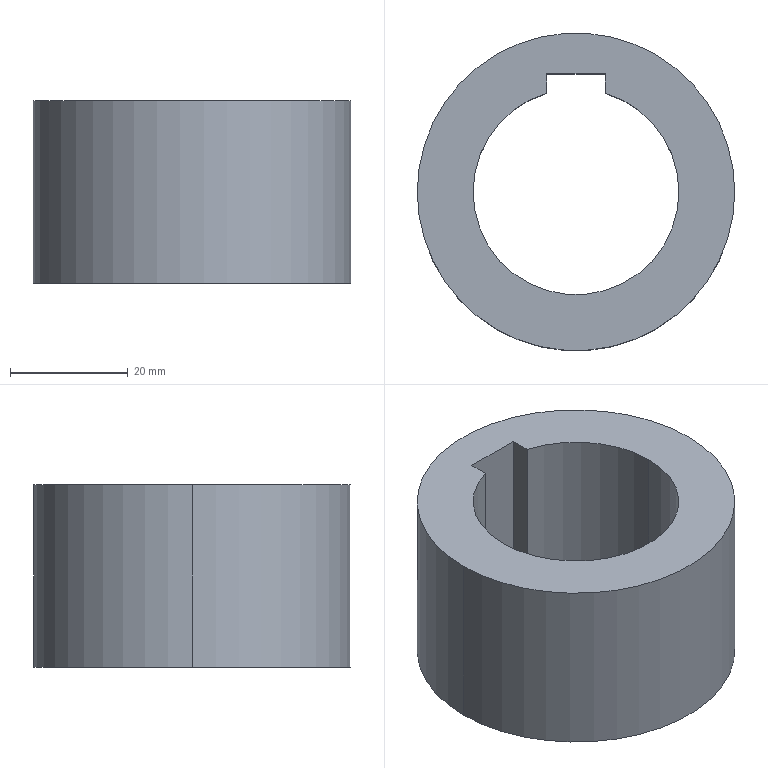Part | SolidWorks | features ICE 3, CirPattern 1, Extrusion 1, RefAxis 1 | 1 solid | 10 faces | box 54 x 54 x 31 mm | volume 40300 mm3 | cylinder 5 | plane 5 | commonest cylinder face diameters 35 x3 54 x2
STEP:
#1=CARTESIAN_POINT('',(-27.,0.,31.));
#2=VERTEX_POINT('',#1);
#3=CARTESIAN_POINT('',(27.,0.,31.));
#4=VERTEX_POINT('',#3);
#5=CARTESIAN_POINT('',(0.,0.,31.));
#6=DIRECTION('',(0.,0.,-1.));
#7=DIRECTION('',(1.,0.,0.));
#8=AXIS2_PLACEMENT_3D('',#5,#6,#7);
#9=CIRCLE('',#8,27.);
#10=EDGE_CURVE('',#2,#4,#9,.T.);
#11=ORIENTED_EDGE('',*,*,#10,.T.);
#12=CARTESIAN_POINT('',(27.,0.,0.));
#13=VERTEX_POINT('',#12);
#14=CARTESIAN_POINT('',(27.,0.,42.));
#15=DIRECTION('',(0.,0.,-1.));
#16=VECTOR('',#15,1000.);
#17=LINE('',#14,#16);
#18=EDGE_CURVE('',#4,#13,#17,.T.);
#19=ORIENTED_EDGE('',*,*,#18,.T.);
#20=CARTESIAN_POINT('',(-27.,0.,0.));
#21=VERTEX_POINT('',#20);
#22=CARTESIAN_POINT('',(0.,0.,0.));
#23=DIRECTION('',(0.,0.,1.));
#24=DIRECTION('',(1.,0.,0.));
#25=AXIS2_PLACEMENT_3D('',#22,#23,#24);
#26=CIRCLE('',#25,27.);
#27=EDGE_CURVE('',#13,#21,#26,.T.);
#28=ORIENTED_EDGE('',*,*,#27,.T.);
#29=CARTESIAN_POINT('',(-27.,0.,42.));
#30=DIRECTION('',(0.,0.,-1.));
#31=VECTOR('',#30,1000.);
#32=LINE('',#29,#31);
#33=EDGE_CURVE('',#2,#21,#32,.T.);
#34=ORIENTED_EDGE('',*,*,#33,.F.);
#35=EDGE_LOOP('',(#11,#19,#28,#34));
#36=FACE_OUTER_BOUND('',#35,.T.);
#37=CARTESIAN_POINT('',(0.,0.,42.));
#38=DIRECTION('',(0.,0.,-1.));
#39=DIRECTION('',(-1.,0.,0.));
#40=AXIS2_PLACEMENT_3D('',#37,#38,#39);
#41=CYLINDRICAL_SURFACE('',#40,27.);
#42=ADVANCED_FACE('',(#36),#41,.T.);
#43=CARTESIAN_POINT('',(-17.5,0.,0.));
#44=VERTEX_POINT('',#43);
#45=CARTESIAN_POINT('',(17.5,0.,0.));
#46=VERTEX_POINT('',#45);
#47=CARTESIAN_POINT('',(0.,0.,0.));
#48=DIRECTION('',(0.,0.,1.));
#49=DIRECTION('',(1.,0.,0.));
#50=AXIS2_PLACEMENT_3D('',#47,#48,#49);
#51=CIRCLE('',#50,17.5);
#52=EDGE_CURVE('',#44,#46,#51,.T.);
#53=ORIENTED_EDGE('',*,*,#52,.F.);
#54=CARTESIAN_POINT('',(-17.5,0.,31.));
#55=VERTEX_POINT('',#54);
#56=CARTESIAN_POINT('',(-17.5,0.,0.));
#57=DIRECTION('',(0.,0.,1.));
#58=VECTOR('',#57,1000.);
#59=LINE('',#56,#58);
#60=EDGE_CURVE('',#44,#55,#59,.T.);
#61=ORIENTED_EDGE('',*,*,#60,.T.);
#62=CARTESIAN_POINT('',(17.5,0.,31.));
#63=VERTEX_POINT('',#62);
#64=CARTESIAN_POINT('',(0.,0.,31.));
#65=DIRECTION('',(0.,0.,1.));
#66=DIRECTION('',(1.,0.,0.));
#67=AXIS2_PLACEMENT_3D('',#64,#65,#66);
#68=CIRCLE('',#67,17.5);
#69=EDGE_CURVE('',#55,#63,#68,.T.);
#70=ORIENTED_EDGE('',*,*,#69,.T.);
#71=CARTESIAN_POINT('',(17.5,0.,0.));
#72=DIRECTION('',(0.,0.,1.));
#73=VECTOR('',#72,1000.);
#74=LINE('',#71,#73);
#75=EDGE_CURVE('',#46,#63,#74,.T.);
#76=ORIENTED_EDGE('',*,*,#75,.F.);
#77=EDGE_LOOP('',(#53,#61,#70,#76));
#78=FACE_OUTER_BOUND('',#77,.T.);
#79=CARTESIAN_POINT('',(0.,0.,0.));
#80=DIRECTION('',(0.,0.,1.));
#81=DIRECTION('',(1.,0.,0.));
#82=AXIS2_PLACEMENT_3D('',#79,#80,#81);
#83=CYLINDRICAL_SURFACE('',#82,17.5);
#84=ADVANCED_FACE('',(#78),#83,.F.);
#85=CARTESIAN_POINT('',(5.,16.771,0.));
#86=VERTEX_POINT('',#85);
#87=CARTESIAN_POINT('',(0.,0.,0.));
#88=DIRECTION('',(0.,0.,1.));
#89=DIRECTION('',(1.,0.,0.));
#90=AXIS2_PLACEMENT_3D('',#87,#88,#89);
#91=CIRCLE('',#90,17.5);
#92=EDGE_CURVE('',#46,#86,#91,.T.);
#93=ORIENTED_EDGE('',*,*,#92,.F.);
#94=ORIENTED_EDGE('',*,*,#75,.T.);
#95=CARTESIAN_POINT('',(5.,16.771,31.));
#96=VERTEX_POINT('',#95);
#97=CARTESIAN_POINT('',(0.,0.,31.));
#98=DIRECTION('',(0.,0.,1.));
#99=DIRECTION('',(1.,0.,0.));
#100=AXIS2_PLACEMENT_3D('',#97,#98,#99);
#101=CIRCLE('',#100,17.5);
#102=EDGE_CURVE('',#63,#96,#101,.T.);
#103=ORIENTED_EDGE('',*,*,#102,.T.);
#104=CARTESIAN_POINT('',(5.,16.771,0.));
#105=DIRECTION('',(0.,0.,1.));
#106=VECTOR('',#105,1000.);
#107=LINE('',#104,#106);
#108=EDGE_CURVE('',#86,#96,#107,.T.);
#109=ORIENTED_EDGE('',*,*,#108,.F.);
#110=EDGE_LOOP('',(#93,#94,#103,#109));
#111=FACE_OUTER_BOUND('',#110,.T.);
#112=CARTESIAN_POINT('',(0.,0.,0.));
#113=DIRECTION('',(0.,0.,1.));
#114=DIRECTION('',(1.,0.,0.));
#115=AXIS2_PLACEMENT_3D('',#112,#113,#114);
#116=CYLINDRICAL_SURFACE('',#115,17.5);
#117=ADVANCED_FACE('',(#111),#116,.F.);
#118=CARTESIAN_POINT('',(-5.,16.771,31.));
#119=VERTEX_POINT('',#118);
#120=CARTESIAN_POINT('',(0.,0.,31.));
#121=DIRECTION('',(0.,0.,1.));
#122=DIRECTION('',(1.,0.,0.));
#123=AXIS2_PLACEMENT_3D('',#120,#121,#122);
#124=CIRCLE('',#123,17.5);
#125=EDGE_CURVE('',#119,#55,#124,.T.);
#126=ORIENTED_EDGE('',*,*,#125,.F.);
#127=CARTESIAN_POINT('',(-5.,20.071,31.));
#128=VERTEX_POINT('',#127);
#129=CARTESIAN_POINT('',(-5.,20.071,31.));
#130=DIRECTION('',(0.,-1.,0.));
#131=VECTOR('',#130,1000.);
#132=LINE('',#129,#131);
#133=EDGE_CURVE('',#128,#119,#132,.T.);
#134=ORIENTED_EDGE('',*,*,#133,.F.);
#135=CARTESIAN_POINT('',(5.,20.071,31.));
#136=VERTEX_POINT('',#135);
#137=CARTESIAN_POINT('',(5.,20.071,31.));
#138=DIRECTION('',(-1.,0.,0.));
#139=VECTOR('',#138,1000.);
#140=LINE('',#137,#139);
#141=EDGE_CURVE('',#136,#128,#140,.T.);
#142=ORIENTED_EDGE('',*,*,#141,.F.);
#143=CARTESIAN_POINT('',(5.,16.771,31.));
#144=DIRECTION('',(0.,1.,0.));
#145=VECTOR('',#144,1000.);
#146=LINE('',#143,#145);
#147=EDGE_CURVE('',#96,#136,#146,.T.);
#148=ORIENTED_EDGE('',*,*,#147,.F.);
#149=ORIENTED_EDGE('',*,*,#102,.F.);
#150=ORIENTED_EDGE('',*,*,#69,.F.);
#151=EDGE_LOOP('',(#126,#134,#142,#148,#149,#150));
#152=FACE_BOUND('',#151,.T.);
#153=ORIENTED_EDGE('',*,*,#10,.F.);
#154=CARTESIAN_POINT('',(0.,0.,31.));
#155=DIRECTION('',(0.,0.,-1.));
#156=DIRECTION('',(1.,0.,0.));
#157=AXIS2_PLACEMENT_3D('',#154,#155,#156);
#158=CIRCLE('',#157,27.);
#159=EDGE_CURVE('',#4,#2,#158,.T.);
#160=ORIENTED_EDGE('',*,*,#159,.F.);
#161=EDGE_LOOP('',(#153,#160));
#162=FACE_OUTER_BOUND('',#161,.T.);
#163=CARTESIAN_POINT('',(0.,0.,31.));
#164=DIRECTION('',(0.,0.,1.));
#165=DIRECTION('',(1.,0.,0.));
#166=AXIS2_PLACEMENT_3D('',#163,#164,#165);
#167=PLANE('',#166);
#168=ADVANCED_FACE('',(#152,#162),#167,.T.);
#169=CARTESIAN_POINT('',(-5.,20.071,0.));
#170=VERTEX_POINT('',#169);
#171=CARTESIAN_POINT('',(-5.,16.771,0.));
#172=VERTEX_POINT('',#171);
#173=CARTESIAN_POINT('',(-5.,20.071,0.));
#174=DIRECTION('',(0.,-1.,0.));
#175=VECTOR('',#174,1000.);
#176=LINE('',#173,#175);
#177=EDGE_CURVE('',#170,#172,#176,.T.);
#178=ORIENTED_EDGE('',*,*,#177,.T.);
#179=CARTESIAN_POINT('',(0.,0.,0.));
#180=DIRECTION('',(0.,0.,1.));
#181=DIRECTION('',(1.,0.,0.));
#182=AXIS2_PLACEMENT_3D('',#179,#180,#181);
#183=CIRCLE('',#182,17.5);
#184=EDGE_CURVE('',#172,#44,#183,.T.);
#185=ORIENTED_EDGE('',*,*,#184,.T.);
#186=ORIENTED_EDGE('',*,*,#52,.T.);
#187=ORIENTED_EDGE('',*,*,#92,.T.);
#188=CARTESIAN_POINT('',(5.,20.071,0.));
#189=VERTEX_POINT('',#188);
#190=CARTESIAN_POINT('',(5.,16.771,0.));
#191=DIRECTION('',(0.,1.,0.));
#192=VECTOR('',#191,1000.);
#193=LINE('',#190,#192);
#194=EDGE_CURVE('',#86,#189,#193,.T.);
#195=ORIENTED_EDGE('',*,*,#194,.T.);
#196=CARTESIAN_POINT('',(5.,20.071,0.));
#197=DIRECTION('',(-1.,0.,0.));
#198=VECTOR('',#197,1000.);
#199=LINE('',#196,#198);
#200=EDGE_CURVE('',#189,#170,#199,.T.);
#201=ORIENTED_EDGE('',*,*,#200,.T.);
#202=EDGE_LOOP('',(#178,#185,#186,#187,#195,#201));
#203=FACE_BOUND('',#202,.T.);
#204=CARTESIAN_POINT('',(0.,0.,0.));
#205=DIRECTION('',(0.,0.,1.));
#206=DIRECTION('',(1.,0.,0.));
#207=AXIS2_PLACEMENT_3D('',#204,#205,#206);
#208=CIRCLE('',#207,27.);
#209=EDGE_CURVE('',#21,#13,#208,.T.);
#210=ORIENTED_EDGE('',*,*,#209,.F.);
#211=ORIENTED_EDGE('',*,*,#27,.F.);
#212=EDGE_LOOP('',(#210,#211));
#213=FACE_OUTER_BOUND('',#212,.T.);
#214=CARTESIAN_POINT('',(0.,0.,0.));
#215=DIRECTION('',(0.,0.,1.));
#216=DIRECTION('',(1.,0.,0.));
#217=AXIS2_PLACEMENT_3D('',#214,#215,#216);
#218=PLANE('',#217);
#219=ADVANCED_FACE('',(#203,#213),#218,.F.);
#220=ORIENTED_EDGE('',*,*,#60,.F.);
#221=ORIENTED_EDGE('',*,*,#184,.F.);
#222=CARTESIAN_POINT('',(-5.,16.771,0.));
#223=DIRECTION('',(0.,0.,1.));
#224=VECTOR('',#223,1000.);
#225=LINE('',#222,#224);
#226=EDGE_CURVE('',#172,#119,#225,.T.);
#227=ORIENTED_EDGE('',*,*,#226,.T.);
#228=ORIENTED_EDGE('',*,*,#125,.T.);
#229=EDGE_LOOP('',(#220,#221,#227,#228));
#230=FACE_OUTER_BOUND('',#229,.T.);
#231=CARTESIAN_POINT('',(0.,0.,0.));
#232=DIRECTION('',(0.,0.,1.));
#233=DIRECTION('',(1.,0.,0.));
#234=AXIS2_PLACEMENT_3D('',#231,#232,#233);
#235=CYLINDRICAL_SURFACE('',#234,17.5);
#236=ADVANCED_FACE('',(#230),#235,.F.);
#237=ORIENTED_EDGE('',*,*,#133,.T.);
#238=ORIENTED_EDGE('',*,*,#226,.F.);
#239=ORIENTED_EDGE('',*,*,#177,.F.);
#240=CARTESIAN_POINT('',(-5.,20.071,0.));
#241=DIRECTION('',(0.,0.,1.));
#242=VECTOR('',#241,1000.);
#243=LINE('',#240,#242);
#244=EDGE_CURVE('',#170,#128,#243,.T.);
#245=ORIENTED_EDGE('',*,*,#244,.T.);
#246=EDGE_LOOP('',(#237,#238,#239,#245));
#247=FACE_OUTER_BOUND('',#246,.T.);
#248=CARTESIAN_POINT('',(-5.,20.071,0.));
#249=DIRECTION('',(-1.,0.,0.));
#250=DIRECTION('',(0.,-1.,0.));
#251=AXIS2_PLACEMENT_3D('',#248,#249,#250);
#252=PLANE('',#251);
#253=ADVANCED_FACE('',(#247),#252,.F.);
#254=ORIENTED_EDGE('',*,*,#141,.T.);
#255=ORIENTED_EDGE('',*,*,#244,.F.);
#256=ORIENTED_EDGE('',*,*,#200,.F.);
#257=CARTESIAN_POINT('',(5.,20.071,0.));
#258=DIRECTION('',(0.,0.,1.));
#259=VECTOR('',#258,1000.);
#260=LINE('',#257,#259);
#261=EDGE_CURVE('',#189,#136,#260,.T.);
#262=ORIENTED_EDGE('',*,*,#261,.T.);
#263=EDGE_LOOP('',(#254,#255,#256,#262));
#264=FACE_OUTER_BOUND('',#263,.T.);
#265=CARTESIAN_POINT('',(5.,20.071,0.));
#266=DIRECTION('',(0.,1.,0.));
#267=DIRECTION('',(0.,0.,1.));
#268=AXIS2_PLACEMENT_3D('',#265,#266,#267);
#269=PLANE('',#268);
#270=ADVANCED_FACE('',(#264),#269,.F.);
#271=ORIENTED_EDGE('',*,*,#147,.T.);
#272=ORIENTED_EDGE('',*,*,#261,.F.);
#273=ORIENTED_EDGE('',*,*,#194,.F.);
#274=ORIENTED_EDGE('',*,*,#108,.T.);
#275=EDGE_LOOP('',(#271,#272,#273,#274));
#276=FACE_OUTER_BOUND('',#275,.T.);
#277=CARTESIAN_POINT('',(5.,16.771,0.));
#278=DIRECTION('',(1.,0.,0.));
#279=DIRECTION('',(0.,1.,0.));
#280=AXIS2_PLACEMENT_3D('',#277,#278,#279);
#281=PLANE('',#280);
#282=ADVANCED_FACE('',(#276),#281,.F.);
#283=ORIENTED_EDGE('',*,*,#18,.F.);
#284=ORIENTED_EDGE('',*,*,#159,.T.);
#285=ORIENTED_EDGE('',*,*,#33,.T.);
#286=ORIENTED_EDGE('',*,*,#209,.T.);
#287=EDGE_LOOP('',(#283,#284,#285,#286));
#288=FACE_OUTER_BOUND('',#287,.T.);
#289=CARTESIAN_POINT('',(0.,0.,42.));
#290=DIRECTION('',(0.,0.,-1.));
#291=DIRECTION('',(-1.,0.,0.));
#292=AXIS2_PLACEMENT_3D('',#289,#290,#291);
#293=CYLINDRICAL_SURFACE('',#292,27.);
#294=ADVANCED_FACE('',(#288),#293,.T.);
#295=CLOSED_SHELL('',(#42,#84,#117,#168,#219,#236,#253,#270,#282,#294));
#296=MANIFOLD_SOLID_BREP('',#295);
#297=CARTESIAN_POINT('',(0.,0.,0.));
#298=DIRECTION('',(0.,0.,1.));
#299=DIRECTION('',(1.,0.,0.));
#300=AXIS2_PLACEMENT_3D('',#297,#298,#299);
#301=(LENGTH_UNIT()NAMED_UNIT(*)SI_UNIT(.MILLI.,.METRE.));
#302=UNCERTAINTY_MEASURE_WITH_UNIT(LENGTH_MEASURE(0.00001),#301,'','');
#303=(NAMED_UNIT(*)PLANE_ANGLE_UNIT()SI_UNIT($,.RADIAN.));
#304=(NAMED_UNIT(*)SI_UNIT($,.STERADIAN.)SOLID_ANGLE_UNIT());
#305=(GEOMETRIC_REPRESENTATION_CONTEXT(3)GLOBAL_UNCERTAINTY_ASSIGNED_CONTEXT((#302))GLOBAL_UNIT_ASSIGNED_CONTEXT((#301,#303,#304))REPRESENTATION_CONTEXT('',''));
#306=ADVANCED_BREP_SHAPE_REPRESENTATION('',(#296,#300),#305);